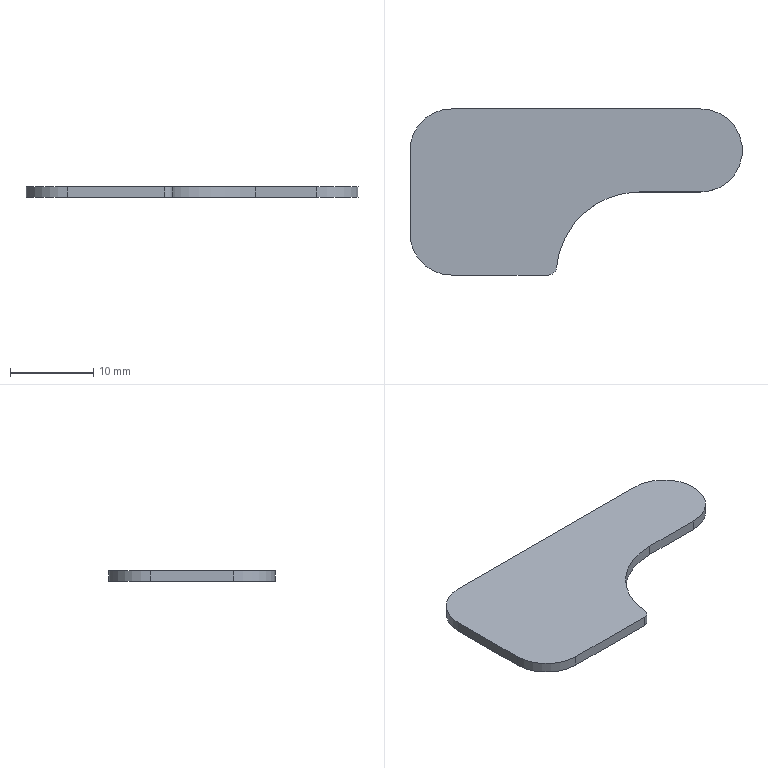Part | STEP file | gslz 2016.10.28-13_id1174_x_t | 1 solid | 11 faces | box 40 x 20 x 1.25 mm | volume 719.671 mm3 | plane 6 | cylinder 5 | commonest cylinder face diameters 10 x3 2 x1 20 x1
STEP:
#1=CARTESIAN_POINT('',(0.,0.,0.));
#2=DIRECTION('',(0.,0.,1.));
#3=DIRECTION('',(1.,0.,0.));
#4=AXIS2_PLACEMENT_3D('',#1,#2,#3);
#5=CARTESIAN_POINT('',(-1119.707,29.496,1.25));
#6=VERTEX_POINT('',#5);
#7=CARTESIAN_POINT('',(-1119.707,39.496,1.25));
#8=VERTEX_POINT('',#7);
#9=CARTESIAN_POINT('',(-1119.707,34.496,1.25));
#10=DIRECTION('',(0.,0.,1.));
#11=DIRECTION('',(-1.,0.,0.));
#12=AXIS2_PLACEMENT_3D('',#9,#10,#11);
#13=CIRCLE('',#12,5.);
#14=CARTESIAN_POINT('',(-346.108,261.5,1.25));
#15=DIRECTION('',(0.,0.,-1.));
#16=DIRECTION('',(-1.,0.,0.));
#17=AXIS2_PLACEMENT_3D('',#14,#15,#16);
#18=PLANE('',#17);
#19=CARTESIAN_POINT('',(778.599,-227.004));
#20=CARTESIAN_POINT('',(778.599,-235.664));
#21=CARTESIAN_POINT('',(771.099,-231.334));
#22=CARTESIAN_POINT('',(763.599,-227.004));
#23=CARTESIAN_POINT('',(771.099,-222.674));
#24=CARTESIAN_POINT('',(778.599,-218.344));
#25=CARTESIAN_POINT('',(778.599,-227.004));
#26=(BOUNDED_CURVE()B_SPLINE_CURVE(2,(#19,#20,#21,#22,#23,#24,#25),.UNSPECIFIED.,.T.,.F.)B_SPLINE_CURVE_WITH_KNOTS((1,2,2,2,2,1),(-2.094,0.,2.094,4.189,6.283,8.378),.UNSPECIFIED.)CURVE()GEOMETRIC_REPRESENTATION_ITEM()RATIONAL_B_SPLINE_CURVE((1.,0.5,1.,0.5,1.,0.5,1.))REPRESENTATION_ITEM(''));
#27=(GEOMETRIC_REPRESENTATION_CONTEXT(2)PARAMETRIC_REPRESENTATION_CONTEXT()REPRESENTATION_CONTEXT('',''));
#28=DEFINITIONAL_REPRESENTATION('',(#26),#27);
#29=PCURVE('',#18,#28);
#30=CARTESIAN_POINT('',(-1119.707,34.496,-2.574));
#31=DIRECTION('',(0.,0.,1.));
#32=DIRECTION('',(1.,0.,0.));
#33=AXIS2_PLACEMENT_3D('',#30,#31,#32);
#34=CYLINDRICAL_SURFACE('',#33,5.);
#35=CARTESIAN_POINT('',(3.142,3.824));
#36=DIRECTION('',(1.,0.));
#37=VECTOR('',#36,1.);
#38=LINE('',#35,#37);
#39=(GEOMETRIC_REPRESENTATION_CONTEXT(2)PARAMETRIC_REPRESENTATION_CONTEXT()REPRESENTATION_CONTEXT('',''));
#40=DEFINITIONAL_REPRESENTATION('',(#38),#39);
#41=PCURVE('',#34,#40);
#42=SURFACE_CURVE('',#13,(#29,#41),.PCURVE_S1.);
#43=EDGE_CURVE('',#6,#8,#42,.T.);
#44=ORIENTED_EDGE('',*,*,#43,.T.);
#45=CARTESIAN_POINT('',(-1149.707,39.496,1.25));
#46=VERTEX_POINT('',#45);
#47=CARTESIAN_POINT('',(-346.108,39.496,1.25));
#48=DIRECTION('',(1.,0.,0.));
#49=VECTOR('',#48,1.);
#50=LINE('',#47,#49);
#51=CARTESIAN_POINT('',(0.,-222.004));
#52=DIRECTION('',(-1.,0.));
#53=VECTOR('',#52,1.);
#54=LINE('',#51,#53);
#55=(GEOMETRIC_REPRESENTATION_CONTEXT(2)PARAMETRIC_REPRESENTATION_CONTEXT()REPRESENTATION_CONTEXT('',''));
#56=DEFINITIONAL_REPRESENTATION('',(#54),#55);
#57=PCURVE('',#18,#56);
#58=CARTESIAN_POINT('',(-1149.707,39.496,-2.574));
#59=DIRECTION('',(0.,-1.,0.));
#60=DIRECTION('',(0.,0.,-1.));
#61=AXIS2_PLACEMENT_3D('',#58,#59,#60);
#62=PLANE('',#61);
#63=CARTESIAN_POINT('',(-3.824,803.599));
#64=DIRECTION('',(0.,1.));
#65=VECTOR('',#64,1.);
#66=LINE('',#63,#65);
#67=(GEOMETRIC_REPRESENTATION_CONTEXT(2)PARAMETRIC_REPRESENTATION_CONTEXT()REPRESENTATION_CONTEXT('',''));
#68=DEFINITIONAL_REPRESENTATION('',(#66),#67);
#69=PCURVE('',#62,#68);
#70=SURFACE_CURVE('',#50,(#57,#69),.PCURVE_S1.);
#71=EDGE_CURVE('',#46,#8,#70,.T.);
#72=ORIENTED_EDGE('',*,*,#71,.F.);
#73=CARTESIAN_POINT('',(-1154.707,34.496,1.25));
#74=VERTEX_POINT('',#73);
#75=CARTESIAN_POINT('',(-1149.707,34.496,1.25));
#76=DIRECTION('',(0.,0.,1.));
#77=DIRECTION('',(-1.,0.,0.));
#78=AXIS2_PLACEMENT_3D('',#75,#76,#77);
#79=CIRCLE('',#78,5.);
#80=CARTESIAN_POINT('',(808.599,-227.004));
#81=CARTESIAN_POINT('',(808.599,-235.664));
#82=CARTESIAN_POINT('',(801.099,-231.334));
#83=CARTESIAN_POINT('',(793.599,-227.004));
#84=CARTESIAN_POINT('',(801.099,-222.674));
#85=CARTESIAN_POINT('',(808.599,-218.344));
#86=CARTESIAN_POINT('',(808.599,-227.004));
#87=(BOUNDED_CURVE()B_SPLINE_CURVE(2,(#80,#81,#82,#83,#84,#85,#86),.UNSPECIFIED.,.T.,.F.)B_SPLINE_CURVE_WITH_KNOTS((1,2,2,2,2,1),(-2.094,0.,2.094,4.189,6.283,8.378),.UNSPECIFIED.)CURVE()GEOMETRIC_REPRESENTATION_ITEM()RATIONAL_B_SPLINE_CURVE((1.,0.5,1.,0.5,1.,0.5,1.))REPRESENTATION_ITEM(''));
#88=(GEOMETRIC_REPRESENTATION_CONTEXT(2)PARAMETRIC_REPRESENTATION_CONTEXT()REPRESENTATION_CONTEXT('',''));
#89=DEFINITIONAL_REPRESENTATION('',(#87),#88);
#90=PCURVE('',#18,#89);
#91=CARTESIAN_POINT('',(-1149.707,34.496,-2.574));
#92=DIRECTION('',(0.,0.,1.));
#93=DIRECTION('',(1.,0.,0.));
#94=AXIS2_PLACEMENT_3D('',#91,#92,#93);
#95=CYLINDRICAL_SURFACE('',#94,5.);
#96=CARTESIAN_POINT('',(-3.142,3.824));
#97=DIRECTION('',(1.,0.));
#98=VECTOR('',#97,1.);
#99=LINE('',#96,#98);
#100=(GEOMETRIC_REPRESENTATION_CONTEXT(2)PARAMETRIC_REPRESENTATION_CONTEXT()REPRESENTATION_CONTEXT('',''));
#101=DEFINITIONAL_REPRESENTATION('',(#99),#100);
#102=PCURVE('',#95,#101);
#103=SURFACE_CURVE('',#79,(#90,#102),.PCURVE_S1.);
#104=EDGE_CURVE('',#46,#74,#103,.T.);
#105=ORIENTED_EDGE('',*,*,#104,.T.);
#106=CARTESIAN_POINT('',(-1154.707,24.496,1.25));
#107=VERTEX_POINT('',#106);
#108=CARTESIAN_POINT('',(-1154.707,261.5,1.25));
#109=DIRECTION('',(0.,1.,0.));
#110=VECTOR('',#109,1.);
#111=LINE('',#108,#110);
#112=CARTESIAN_POINT('',(808.599,0.));
#113=DIRECTION('',(0.,1.));
#114=VECTOR('',#113,1.);
#115=LINE('',#112,#114);
#116=(GEOMETRIC_REPRESENTATION_CONTEXT(2)PARAMETRIC_REPRESENTATION_CONTEXT()REPRESENTATION_CONTEXT('',''));
#117=DEFINITIONAL_REPRESENTATION('',(#115),#116);
#118=PCURVE('',#18,#117);
#119=CARTESIAN_POINT('',(-1154.707,24.496,-2.574));
#120=DIRECTION('',(1.,0.,0.));
#121=DIRECTION('',(0.,0.,-1.));
#122=AXIS2_PLACEMENT_3D('',#119,#120,#121);
#123=PLANE('',#122);
#124=CARTESIAN_POINT('',(-3.824,237.004));
#125=DIRECTION('',(0.,1.));
#126=VECTOR('',#125,1.);
#127=LINE('',#124,#126);
#128=(GEOMETRIC_REPRESENTATION_CONTEXT(2)PARAMETRIC_REPRESENTATION_CONTEXT()REPRESENTATION_CONTEXT('',''));
#129=DEFINITIONAL_REPRESENTATION('',(#127),#128);
#130=PCURVE('',#123,#129);
#131=SURFACE_CURVE('',#111,(#118,#130),.PCURVE_S1.);
#132=EDGE_CURVE('',#107,#74,#131,.T.);
#133=ORIENTED_EDGE('',*,*,#132,.F.);
#134=CARTESIAN_POINT('',(-1149.707,19.496,1.25));
#135=VERTEX_POINT('',#134);
#136=CARTESIAN_POINT('',(-1149.707,24.496,1.25));
#137=DIRECTION('',(0.,0.,1.));
#138=DIRECTION('',(-1.,0.,0.));
#139=AXIS2_PLACEMENT_3D('',#136,#137,#138);
#140=CIRCLE('',#139,5.);
#141=CARTESIAN_POINT('',(808.599,-237.004));
#142=CARTESIAN_POINT('',(808.599,-245.664));
#143=CARTESIAN_POINT('',(801.099,-241.334));
#144=CARTESIAN_POINT('',(793.599,-237.004));
#145=CARTESIAN_POINT('',(801.099,-232.674));
#146=CARTESIAN_POINT('',(808.599,-228.344));
#147=CARTESIAN_POINT('',(808.599,-237.004));
#148=(BOUNDED_CURVE()B_SPLINE_CURVE(2,(#141,#142,#143,#144,#145,#146,#147),.UNSPECIFIED.,.T.,.F.)B_SPLINE_CURVE_WITH_KNOTS((1,2,2,2,2,1),(-2.094,0.,2.094,4.189,6.283,8.378),.UNSPECIFIED.)CURVE()GEOMETRIC_REPRESENTATION_ITEM()RATIONAL_B_SPLINE_CURVE((1.,0.5,1.,0.5,1.,0.5,1.))REPRESENTATION_ITEM(''));
#149=(GEOMETRIC_REPRESENTATION_CONTEXT(2)PARAMETRIC_REPRESENTATION_CONTEXT()REPRESENTATION_CONTEXT('',''));
#150=DEFINITIONAL_REPRESENTATION('',(#148),#149);
#151=PCURVE('',#18,#150);
#152=CARTESIAN_POINT('',(-1149.707,24.496,-2.574));
#153=DIRECTION('',(0.,0.,1.));
#154=DIRECTION('',(1.,0.,0.));
#155=AXIS2_PLACEMENT_3D('',#152,#153,#154);
#156=CYLINDRICAL_SURFACE('',#155,5.);
#157=CARTESIAN_POINT('',(3.142,3.824));
#158=DIRECTION('',(1.,0.));
#159=VECTOR('',#158,1.);
#160=LINE('',#157,#159);
#161=(GEOMETRIC_REPRESENTATION_CONTEXT(2)PARAMETRIC_REPRESENTATION_CONTEXT()REPRESENTATION_CONTEXT('',''));
#162=DEFINITIONAL_REPRESENTATION('',(#160),#161);
#163=PCURVE('',#156,#162);
#164=SURFACE_CURVE('',#140,(#151,#163),.PCURVE_S1.);
#165=EDGE_CURVE('',#107,#135,#164,.T.);
#166=ORIENTED_EDGE('',*,*,#165,.T.);
#167=CARTESIAN_POINT('',(-1138.069,19.496,1.25));
#168=VERTEX_POINT('',#167);
#169=CARTESIAN_POINT('',(-346.108,19.496,1.25));
#170=DIRECTION('',(1.,0.,0.));
#171=VECTOR('',#170,1.);
#172=LINE('',#169,#171);
#173=CARTESIAN_POINT('',(0.,-242.004));
#174=DIRECTION('',(-1.,0.));
#175=VECTOR('',#174,1.);
#176=LINE('',#173,#175);
#177=(GEOMETRIC_REPRESENTATION_CONTEXT(2)PARAMETRIC_REPRESENTATION_CONTEXT()REPRESENTATION_CONTEXT('',''));
#178=DEFINITIONAL_REPRESENTATION('',(#176),#177);
#179=PCURVE('',#18,#178);
#180=CARTESIAN_POINT('',(-1141.069,19.496,-2.574));
#181=DIRECTION('',(0.,1.,0.));
#182=DIRECTION('',(0.,0.,1.));
#183=AXIS2_PLACEMENT_3D('',#180,#181,#182);
#184=PLANE('',#183);
#185=CARTESIAN_POINT('',(3.824,794.961));
#186=DIRECTION('',(0.,1.));
#187=VECTOR('',#186,1.);
#188=LINE('',#185,#187);
#189=(GEOMETRIC_REPRESENTATION_CONTEXT(2)PARAMETRIC_REPRESENTATION_CONTEXT()REPRESENTATION_CONTEXT('',''));
#190=DEFINITIONAL_REPRESENTATION('',(#188),#189);
#191=PCURVE('',#184,#190);
#192=SURFACE_CURVE('',#172,(#179,#191),.PCURVE_S1.);
#193=EDGE_CURVE('',#135,#168,#192,.T.);
#194=ORIENTED_EDGE('',*,*,#193,.T.);
#195=CARTESIAN_POINT('',(-1137.073,20.405,1.25));
#196=VERTEX_POINT('',#195);
#197=CARTESIAN_POINT('',(-1138.069,20.496,1.25));
#198=DIRECTION('',(0.,0.,1.));
#199=DIRECTION('',(-1.,0.,0.));
#200=AXIS2_PLACEMENT_3D('',#197,#198,#199);
#201=CIRCLE('',#200,1.);
#202=CARTESIAN_POINT('',(792.961,-241.004));
#203=CARTESIAN_POINT('',(792.961,-242.736));
#204=CARTESIAN_POINT('',(791.461,-241.87));
#205=CARTESIAN_POINT('',(789.961,-241.004));
#206=CARTESIAN_POINT('',(791.461,-240.138));
#207=CARTESIAN_POINT('',(792.961,-239.272));
#208=CARTESIAN_POINT('',(792.961,-241.004));
#209=(BOUNDED_CURVE()B_SPLINE_CURVE(2,(#202,#203,#204,#205,#206,#207,#208),.UNSPECIFIED.,.T.,.F.)B_SPLINE_CURVE_WITH_KNOTS((1,2,2,2,2,1),(-2.094,0.,2.094,4.189,6.283,8.378),.UNSPECIFIED.)CURVE()GEOMETRIC_REPRESENTATION_ITEM()RATIONAL_B_SPLINE_CURVE((1.,0.5,1.,0.5,1.,0.5,1.))REPRESENTATION_ITEM(''));
#210=(GEOMETRIC_REPRESENTATION_CONTEXT(2)PARAMETRIC_REPRESENTATION_CONTEXT()REPRESENTATION_CONTEXT('',''));
#211=DEFINITIONAL_REPRESENTATION('',(#209),#210);
#212=PCURVE('',#18,#211);
#213=CARTESIAN_POINT('',(-1138.069,20.496,-2.574));
#214=DIRECTION('',(0.,0.,1.));
#215=DIRECTION('',(1.,0.,0.));
#216=AXIS2_PLACEMENT_3D('',#213,#214,#215);
#217=CYLINDRICAL_SURFACE('',#216,1.);
#218=CARTESIAN_POINT('',(3.142,3.824));
#219=DIRECTION('',(1.,0.));
#220=VECTOR('',#219,1.);
#221=LINE('',#218,#220);
#222=(GEOMETRIC_REPRESENTATION_CONTEXT(2)PARAMETRIC_REPRESENTATION_CONTEXT()REPRESENTATION_CONTEXT('',''));
#223=DEFINITIONAL_REPRESENTATION('',(#221),#222);
#224=PCURVE('',#217,#223);
#225=SURFACE_CURVE('',#201,(#212,#224),.PCURVE_S1.);
#226=EDGE_CURVE('',#168,#196,#225,.T.);
#227=ORIENTED_EDGE('',*,*,#226,.T.);
#228=CARTESIAN_POINT('',(-1127.115,29.496,1.25));
#229=VERTEX_POINT('',#228);
#230=CARTESIAN_POINT('',(-1127.115,19.496,1.25));
#231=DIRECTION('',(0.,0.,-1.));
#232=DIRECTION('',(-1.,0.,0.));
#233=AXIS2_PLACEMENT_3D('',#230,#231,#232);
#234=CIRCLE('',#233,10.);
#235=CARTESIAN_POINT('',(781.007,-242.004));
#236=DIRECTION('',(1.,0.));
#237=AXIS2_PLACEMENT_2D('',#235,#236);
#238=CIRCLE('',#237,10.);
#239=(GEOMETRIC_REPRESENTATION_CONTEXT(2)PARAMETRIC_REPRESENTATION_CONTEXT()REPRESENTATION_CONTEXT('',''));
#240=DEFINITIONAL_REPRESENTATION('',(#238),#239);
#241=PCURVE('',#18,#240);
#242=CARTESIAN_POINT('',(-1127.115,19.496,-2.574));
#243=DIRECTION('',(0.,0.,1.));
#244=DIRECTION('',(1.,0.,0.));
#245=AXIS2_PLACEMENT_3D('',#242,#243,#244);
#246=CYLINDRICAL_SURFACE('',#245,10.);
#247=CARTESIAN_POINT('',(3.142,3.824));
#248=DIRECTION('',(-1.,0.));
#249=VECTOR('',#248,1.);
#250=LINE('',#247,#249);
#251=(GEOMETRIC_REPRESENTATION_CONTEXT(2)PARAMETRIC_REPRESENTATION_CONTEXT()REPRESENTATION_CONTEXT('',''));
#252=DEFINITIONAL_REPRESENTATION('',(#250),#251);
#253=PCURVE('',#246,#252);
#254=SURFACE_CURVE('',#234,(#241,#253),.PCURVE_S1.);
#255=EDGE_CURVE('',#196,#229,#254,.T.);
#256=ORIENTED_EDGE('',*,*,#255,.T.);
#257=CARTESIAN_POINT('',(-346.108,29.496,1.25));
#258=DIRECTION('',(-1.,0.,0.));
#259=VECTOR('',#258,1.);
#260=LINE('',#257,#259);
#261=CARTESIAN_POINT('',(0.,-232.004));
#262=DIRECTION('',(1.,0.));
#263=VECTOR('',#262,1.);
#264=LINE('',#261,#263);
#265=(GEOMETRIC_REPRESENTATION_CONTEXT(2)PARAMETRIC_REPRESENTATION_CONTEXT()REPRESENTATION_CONTEXT('',''));
#266=DEFINITIONAL_REPRESENTATION('',(#264),#265);
#267=PCURVE('',#18,#266);
#268=CARTESIAN_POINT('',(-1119.707,29.496,-2.574));
#269=DIRECTION('',(0.,1.,0.));
#270=DIRECTION('',(-1.,0.,0.));
#271=AXIS2_PLACEMENT_3D('',#268,#269,#270);
#272=PLANE('',#271);
#273=CARTESIAN_POINT('',(-773.599,3.824));
#274=DIRECTION('',(1.,0.));
#275=VECTOR('',#274,1.);
#276=LINE('',#273,#275);
#277=(GEOMETRIC_REPRESENTATION_CONTEXT(2)PARAMETRIC_REPRESENTATION_CONTEXT()REPRESENTATION_CONTEXT('',''));
#278=DEFINITIONAL_REPRESENTATION('',(#276),#277);
#279=PCURVE('',#272,#278);
#280=SURFACE_CURVE('',#260,(#267,#279),.PCURVE_S1.);
#281=EDGE_CURVE('',#6,#229,#280,.T.);
#282=ORIENTED_EDGE('',*,*,#281,.F.);
#283=EDGE_LOOP('',(#44,#72,#105,#133,#166,#194,#227,#256,#282));
#284=FACE_BOUND('',#283,.T.);
#285=ADVANCED_FACE('',(#284),#18,.F.);
#286=CARTESIAN_POINT('',(-1119.707,39.496,0.));
#287=VERTEX_POINT('',#286);
#288=CARTESIAN_POINT('',(-1149.707,39.496,0.));
#289=VERTEX_POINT('',#288);
#290=CARTESIAN_POINT('',(-346.108,39.496,0.));
#291=DIRECTION('',(-1.,0.,0.));
#292=VECTOR('',#291,1.);
#293=LINE('',#290,#292);
#294=CARTESIAN_POINT('',(-2.574,803.599));
#295=DIRECTION('',(0.,-1.));
#296=VECTOR('',#295,1.);
#297=LINE('',#294,#296);
#298=(GEOMETRIC_REPRESENTATION_CONTEXT(2)PARAMETRIC_REPRESENTATION_CONTEXT()REPRESENTATION_CONTEXT('',''));
#299=DEFINITIONAL_REPRESENTATION('',(#297),#298);
#300=PCURVE('',#62,#299);
#301=CARTESIAN_POINT('',(-346.108,261.5,0.));
#302=DIRECTION('',(0.,0.,-1.));
#303=DIRECTION('',(-1.,0.,0.));
#304=AXIS2_PLACEMENT_3D('',#301,#302,#303);
#305=PLANE('',#304);
#306=CARTESIAN_POINT('',(0.,-222.004));
#307=DIRECTION('',(1.,0.));
#308=VECTOR('',#307,1.);
#309=LINE('',#306,#308);
#310=(GEOMETRIC_REPRESENTATION_CONTEXT(2)PARAMETRIC_REPRESENTATION_CONTEXT()REPRESENTATION_CONTEXT('',''));
#311=DEFINITIONAL_REPRESENTATION('',(#309),#310);
#312=PCURVE('',#305,#311);
#313=SURFACE_CURVE('',#293,(#300,#312),.PCURVE_S1.);
#314=EDGE_CURVE('',#287,#289,#313,.T.);
#315=ORIENTED_EDGE('',*,*,#314,.T.);
#316=CARTESIAN_POINT('',(-1149.707,39.496,-2.574));
#317=DIRECTION('',(0.,0.,-1.));
#318=VECTOR('',#317,1.);
#319=LINE('',#316,#318);
#320=CARTESIAN_POINT('',(0.,0.));
#321=DIRECTION('',(1.,0.));
#322=VECTOR('',#321,1.);
#323=LINE('',#320,#322);
#324=(GEOMETRIC_REPRESENTATION_CONTEXT(2)PARAMETRIC_REPRESENTATION_CONTEXT()REPRESENTATION_CONTEXT('',''));
#325=DEFINITIONAL_REPRESENTATION('',(#323),#324);
#326=PCURVE('',#62,#325);
#327=CARTESIAN_POINT('',(1.571,0.));
#328=DIRECTION('',(0.,-1.));
#329=VECTOR('',#328,1.);
#330=LINE('',#327,#329);
#331=(GEOMETRIC_REPRESENTATION_CONTEXT(2)PARAMETRIC_REPRESENTATION_CONTEXT()REPRESENTATION_CONTEXT('',''));
#332=DEFINITIONAL_REPRESENTATION('',(#330),#331);
#333=PCURVE('',#95,#332);
#334=SURFACE_CURVE('',#319,(#326,#333),.PCURVE_S1.);
#335=EDGE_CURVE('',#46,#289,#334,.T.);
#336=ORIENTED_EDGE('',*,*,#335,.F.);
#337=ORIENTED_EDGE('',*,*,#71,.T.);
#338=CARTESIAN_POINT('',(-1119.707,39.496,-2.574));
#339=DIRECTION('',(0.,0.,-1.));
#340=VECTOR('',#339,1.);
#341=LINE('',#338,#340);
#342=CARTESIAN_POINT('',(0.,30.));
#343=DIRECTION('',(1.,0.));
#344=VECTOR('',#343,1.);
#345=LINE('',#342,#344);
#346=(GEOMETRIC_REPRESENTATION_CONTEXT(2)PARAMETRIC_REPRESENTATION_CONTEXT()REPRESENTATION_CONTEXT('',''));
#347=DEFINITIONAL_REPRESENTATION('',(#345),#346);
#348=PCURVE('',#62,#347);
#349=CARTESIAN_POINT('',(7.854,0.));
#350=DIRECTION('',(0.,-1.));
#351=VECTOR('',#350,1.);
#352=LINE('',#349,#351);
#353=(GEOMETRIC_REPRESENTATION_CONTEXT(2)PARAMETRIC_REPRESENTATION_CONTEXT()REPRESENTATION_CONTEXT('',''));
#354=DEFINITIONAL_REPRESENTATION('',(#352),#353);
#355=PCURVE('',#34,#354);
#356=SURFACE_CURVE('',#341,(#348,#355),.PCURVE_S1.);
#357=EDGE_CURVE('',#8,#287,#356,.T.);
#358=ORIENTED_EDGE('',*,*,#357,.T.);
#359=EDGE_LOOP('',(#315,#336,#337,#358));
#360=FACE_BOUND('',#359,.T.);
#361=ADVANCED_FACE('',(#360),#62,.F.);
#362=CARTESIAN_POINT('',(-1119.707,29.496,0.));
#363=VERTEX_POINT('',#362);
#364=CARTESIAN_POINT('',(-1119.707,34.496,0.));
#365=DIRECTION('',(0.,0.,1.));
#366=DIRECTION('',(-1.,0.,0.));
#367=AXIS2_PLACEMENT_3D('',#364,#365,#366);
#368=CIRCLE('',#367,5.);
#369=CARTESIAN_POINT('',(3.142,2.574));
#370=DIRECTION('',(1.,0.));
#371=VECTOR('',#370,1.);
#372=LINE('',#369,#371);
#373=(GEOMETRIC_REPRESENTATION_CONTEXT(2)PARAMETRIC_REPRESENTATION_CONTEXT()REPRESENTATION_CONTEXT('',''));
#374=DEFINITIONAL_REPRESENTATION('',(#372),#373);
#375=PCURVE('',#34,#374);
#376=CARTESIAN_POINT('',(778.599,-227.004));
#377=CARTESIAN_POINT('',(778.599,-235.664));
#378=CARTESIAN_POINT('',(771.099,-231.334));
#379=CARTESIAN_POINT('',(763.599,-227.004));
#380=CARTESIAN_POINT('',(771.099,-222.674));
#381=CARTESIAN_POINT('',(778.599,-218.344));
#382=CARTESIAN_POINT('',(778.599,-227.004));
#383=(BOUNDED_CURVE()B_SPLINE_CURVE(2,(#376,#377,#378,#379,#380,#381,#382),.UNSPECIFIED.,.T.,.F.)B_SPLINE_CURVE_WITH_KNOTS((1,2,2,2,2,1),(-2.094,0.,2.094,4.189,6.283,8.378),.UNSPECIFIED.)CURVE()GEOMETRIC_REPRESENTATION_ITEM()RATIONAL_B_SPLINE_CURVE((1.,0.5,1.,0.5,1.,0.5,1.))REPRESENTATION_ITEM(''));
#384=(GEOMETRIC_REPRESENTATION_CONTEXT(2)PARAMETRIC_REPRESENTATION_CONTEXT()REPRESENTATION_CONTEXT('',''));
#385=DEFINITIONAL_REPRESENTATION('',(#383),#384);
#386=PCURVE('',#305,#385);
#387=SURFACE_CURVE('',#368,(#375,#386),.PCURVE_S1.);
#388=EDGE_CURVE('',#363,#287,#387,.T.);
#389=ORIENTED_EDGE('',*,*,#388,.T.);
#390=ORIENTED_EDGE('',*,*,#357,.F.);
#391=ORIENTED_EDGE('',*,*,#43,.F.);
#392=CARTESIAN_POINT('',(-1119.707,29.496,-2.574));
#393=DIRECTION('',(0.,0.,-1.));
#394=VECTOR('',#393,1.);
#395=LINE('',#392,#394);
#396=CARTESIAN_POINT('',(4.712,0.));
#397=DIRECTION('',(0.,-1.));
#398=VECTOR('',#397,1.);
#399=LINE('',#396,#398);
#400=(GEOMETRIC_REPRESENTATION_CONTEXT(2)PARAMETRIC_REPRESENTATION_CONTEXT()REPRESENTATION_CONTEXT('',''));
#401=DEFINITIONAL_REPRESENTATION('',(#399),#400);
#402=PCURVE('',#34,#401);
#403=CARTESIAN_POINT('',(0.,0.));
#404=DIRECTION('',(0.,-1.));
#405=VECTOR('',#404,1.);
#406=LINE('',#403,#405);
#407=(GEOMETRIC_REPRESENTATION_CONTEXT(2)PARAMETRIC_REPRESENTATION_CONTEXT()REPRESENTATION_CONTEXT('',''));
#408=DEFINITIONAL_REPRESENTATION('',(#406),#407);
#409=PCURVE('',#272,#408);
#410=SURFACE_CURVE('',#395,(#402,#409),.PCURVE_S1.);
#411=EDGE_CURVE('',#6,#363,#410,.T.);
#412=ORIENTED_EDGE('',*,*,#411,.T.);
#413=EDGE_LOOP('',(#389,#390,#391,#412));
#414=FACE_BOUND('',#413,.T.);
#415=ADVANCED_FACE('',(#414),#34,.T.);
#416=CARTESIAN_POINT('',(-1127.115,29.496,0.));
#417=VERTEX_POINT('',#416);
#418=CARTESIAN_POINT('',(-346.108,29.496,0.));
#419=DIRECTION('',(-1.,0.,0.));
#420=VECTOR('',#419,1.);
#421=LINE('',#418,#420);
#422=CARTESIAN_POINT('',(-773.599,2.574));
#423=DIRECTION('',(1.,0.));
#424=VECTOR('',#423,1.);
#425=LINE('',#422,#424);
#426=(GEOMETRIC_REPRESENTATION_CONTEXT(2)PARAMETRIC_REPRESENTATION_CONTEXT()REPRESENTATION_CONTEXT('',''));
#427=DEFINITIONAL_REPRESENTATION('',(#425),#426);
#428=PCURVE('',#272,#427);
#429=CARTESIAN_POINT('',(0.,-232.004));
#430=DIRECTION('',(1.,0.));
#431=VECTOR('',#430,1.);
#432=LINE('',#429,#431);
#433=(GEOMETRIC_REPRESENTATION_CONTEXT(2)PARAMETRIC_REPRESENTATION_CONTEXT()REPRESENTATION_CONTEXT('',''));
#434=DEFINITIONAL_REPRESENTATION('',(#432),#433);
#435=PCURVE('',#305,#434);
#436=SURFACE_CURVE('',#421,(#428,#435),.PCURVE_S1.);
#437=EDGE_CURVE('',#363,#417,#436,.T.);
#438=ORIENTED_EDGE('',*,*,#437,.F.);
#439=ORIENTED_EDGE('',*,*,#411,.F.);
#440=ORIENTED_EDGE('',*,*,#281,.T.);
#441=CARTESIAN_POINT('',(-1127.115,29.496,-2.574));
#442=DIRECTION('',(0.,0.,-1.));
#443=VECTOR('',#442,1.);
#444=LINE('',#441,#443);
#445=CARTESIAN_POINT('',(7.408,0.));
#446=DIRECTION('',(0.,-1.));
#447=VECTOR('',#446,1.);
#448=LINE('',#445,#447);
#449=(GEOMETRIC_REPRESENTATION_CONTEXT(2)PARAMETRIC_REPRESENTATION_CONTEXT()REPRESENTATION_CONTEXT('',''));
#450=DEFINITIONAL_REPRESENTATION('',(#448),#449);
#451=PCURVE('',#272,#450);
#452=CARTESIAN_POINT('',(1.571,0.));
#453=DIRECTION('',(0.,-1.));
#454=VECTOR('',#453,1.);
#455=LINE('',#452,#454);
#456=(GEOMETRIC_REPRESENTATION_CONTEXT(2)PARAMETRIC_REPRESENTATION_CONTEXT()REPRESENTATION_CONTEXT('',''));
#457=DEFINITIONAL_REPRESENTATION('',(#455),#456);
#458=PCURVE('',#246,#457);
#459=SURFACE_CURVE('',#444,(#451,#458),.PCURVE_S1.);
#460=EDGE_CURVE('',#229,#417,#459,.T.);
#461=ORIENTED_EDGE('',*,*,#460,.T.);
#462=EDGE_LOOP('',(#438,#439,#440,#461));
#463=FACE_BOUND('',#462,.T.);
#464=ADVANCED_FACE('',(#463),#272,.F.);
#465=CARTESIAN_POINT('',(-1137.073,20.405,0.));
#466=VERTEX_POINT('',#465);
#467=CARTESIAN_POINT('',(-1137.073,20.405,-2.574));
#468=DIRECTION('',(0.,0.,-1.));
#469=VECTOR('',#468,1.);
#470=LINE('',#467,#469);
#471=CARTESIAN_POINT('',(3.051,0.));
#472=DIRECTION('',(0.,-1.));
#473=VECTOR('',#472,1.);
#474=LINE('',#471,#473);
#475=(GEOMETRIC_REPRESENTATION_CONTEXT(2)PARAMETRIC_REPRESENTATION_CONTEXT()REPRESENTATION_CONTEXT('',''));
#476=DEFINITIONAL_REPRESENTATION('',(#474),#475);
#477=PCURVE('',#246,#476);
#478=CARTESIAN_POINT('',(6.192,0.));
#479=DIRECTION('',(0.,-1.));
#480=VECTOR('',#479,1.);
#481=LINE('',#478,#480);
#482=(GEOMETRIC_REPRESENTATION_CONTEXT(2)PARAMETRIC_REPRESENTATION_CONTEXT()REPRESENTATION_CONTEXT('',''));
#483=DEFINITIONAL_REPRESENTATION('',(#481),#482);
#484=PCURVE('',#217,#483);
#485=SURFACE_CURVE('',#470,(#477,#484),.PCURVE_S1.);
#486=EDGE_CURVE('',#196,#466,#485,.T.);
#487=ORIENTED_EDGE('',*,*,#486,.F.);
#488=ORIENTED_EDGE('',*,*,#255,.T.);
#489=ORIENTED_EDGE('',*,*,#460,.T.);
#490=CARTESIAN_POINT('',(-1127.115,19.496,0.));
#491=DIRECTION('',(0.,0.,-1.));
#492=DIRECTION('',(-1.,0.,0.));
#493=AXIS2_PLACEMENT_3D('',#490,#491,#492);
#494=CIRCLE('',#493,10.);
#495=CARTESIAN_POINT('',(3.142,2.574));
#496=DIRECTION('',(-1.,0.));
#497=VECTOR('',#496,1.);
#498=LINE('',#495,#497);
#499=(GEOMETRIC_REPRESENTATION_CONTEXT(2)PARAMETRIC_REPRESENTATION_CONTEXT()REPRESENTATION_CONTEXT('',''));
#500=DEFINITIONAL_REPRESENTATION('',(#498),#499);
#501=PCURVE('',#246,#500);
#502=CARTESIAN_POINT('',(781.007,-242.004));
#503=DIRECTION('',(1.,0.));
#504=AXIS2_PLACEMENT_2D('',#502,#503);
#505=CIRCLE('',#504,10.);
#506=(GEOMETRIC_REPRESENTATION_CONTEXT(2)PARAMETRIC_REPRESENTATION_CONTEXT()REPRESENTATION_CONTEXT('',''));
#507=DEFINITIONAL_REPRESENTATION('',(#505),#506);
#508=PCURVE('',#305,#507);
#509=SURFACE_CURVE('',#494,(#501,#508),.PCURVE_S1.);
#510=EDGE_CURVE('',#466,#417,#509,.T.);
#511=ORIENTED_EDGE('',*,*,#510,.F.);
#512=EDGE_LOOP('',(#487,#488,#489,#511));
#513=FACE_BOUND('',#512,.F.);
#514=ADVANCED_FACE('',(#513),#246,.F.);
#515=CARTESIAN_POINT('',(-1138.069,19.496,0.));
#516=VERTEX_POINT('',#515);
#517=CARTESIAN_POINT('',(-1138.069,20.496,0.));
#518=DIRECTION('',(0.,0.,1.));
#519=DIRECTION('',(-1.,0.,0.));
#520=AXIS2_PLACEMENT_3D('',#517,#518,#519);
#521=CIRCLE('',#520,1.);
#522=CARTESIAN_POINT('',(3.142,2.574));
#523=DIRECTION('',(1.,0.));
#524=VECTOR('',#523,1.);
#525=LINE('',#522,#524);
#526=(GEOMETRIC_REPRESENTATION_CONTEXT(2)PARAMETRIC_REPRESENTATION_CONTEXT()REPRESENTATION_CONTEXT('',''));
#527=DEFINITIONAL_REPRESENTATION('',(#525),#526);
#528=PCURVE('',#217,#527);
#529=CARTESIAN_POINT('',(792.961,-241.004));
#530=CARTESIAN_POINT('',(792.961,-242.736));
#531=CARTESIAN_POINT('',(791.461,-241.87));
#532=CARTESIAN_POINT('',(789.961,-241.004));
#533=CARTESIAN_POINT('',(791.461,-240.138));
#534=CARTESIAN_POINT('',(792.961,-239.272));
#535=CARTESIAN_POINT('',(792.961,-241.004));
#536=(BOUNDED_CURVE()B_SPLINE_CURVE(2,(#529,#530,#531,#532,#533,#534,#535),.UNSPECIFIED.,.T.,.F.)B_SPLINE_CURVE_WITH_KNOTS((1,2,2,2,2,1),(-2.094,0.,2.094,4.189,6.283,8.378),.UNSPECIFIED.)CURVE()GEOMETRIC_REPRESENTATION_ITEM()RATIONAL_B_SPLINE_CURVE((1.,0.5,1.,0.5,1.,0.5,1.))REPRESENTATION_ITEM(''));
#537=(GEOMETRIC_REPRESENTATION_CONTEXT(2)PARAMETRIC_REPRESENTATION_CONTEXT()REPRESENTATION_CONTEXT('',''));
#538=DEFINITIONAL_REPRESENTATION('',(#536),#537);
#539=PCURVE('',#305,#538);
#540=SURFACE_CURVE('',#521,(#528,#539),.PCURVE_S1.);
#541=EDGE_CURVE('',#516,#466,#540,.T.);
#542=ORIENTED_EDGE('',*,*,#541,.T.);
#543=ORIENTED_EDGE('',*,*,#486,.F.);
#544=ORIENTED_EDGE('',*,*,#226,.F.);
#545=CARTESIAN_POINT('',(-1138.069,19.496,-2.574));
#546=DIRECTION('',(0.,0.,-1.));
#547=VECTOR('',#546,1.);
#548=LINE('',#545,#547);
#549=CARTESIAN_POINT('',(4.712,0.));
#550=DIRECTION('',(0.,-1.));
#551=VECTOR('',#550,1.);
#552=LINE('',#549,#551);
#553=(GEOMETRIC_REPRESENTATION_CONTEXT(2)PARAMETRIC_REPRESENTATION_CONTEXT()REPRESENTATION_CONTEXT('',''));
#554=DEFINITIONAL_REPRESENTATION('',(#552),#553);
#555=PCURVE('',#217,#554);
#556=CARTESIAN_POINT('',(0.,3.));
#557=DIRECTION('',(-1.,0.));
#558=VECTOR('',#557,1.);
#559=LINE('',#556,#558);
#560=(GEOMETRIC_REPRESENTATION_CONTEXT(2)PARAMETRIC_REPRESENTATION_CONTEXT()REPRESENTATION_CONTEXT('',''));
#561=DEFINITIONAL_REPRESENTATION('',(#559),#560);
#562=PCURVE('',#184,#561);
#563=SURFACE_CURVE('',#548,(#555,#562),.PCURVE_S1.);
#564=EDGE_CURVE('',#168,#516,#563,.T.);
#565=ORIENTED_EDGE('',*,*,#564,.T.);
#566=EDGE_LOOP('',(#542,#543,#544,#565));
#567=FACE_BOUND('',#566,.T.);
#568=ADVANCED_FACE('',(#567),#217,.T.);
#569=CARTESIAN_POINT('',(-1149.707,19.496,0.));
#570=VERTEX_POINT('',#569);
#571=CARTESIAN_POINT('',(-346.108,19.496,0.));
#572=DIRECTION('',(1.,0.,0.));
#573=VECTOR('',#572,1.);
#574=LINE('',#571,#573);
#575=CARTESIAN_POINT('',(2.574,794.961));
#576=DIRECTION('',(0.,1.));
#577=VECTOR('',#576,1.);
#578=LINE('',#575,#577);
#579=(GEOMETRIC_REPRESENTATION_CONTEXT(2)PARAMETRIC_REPRESENTATION_CONTEXT()REPRESENTATION_CONTEXT('',''));
#580=DEFINITIONAL_REPRESENTATION('',(#578),#579);
#581=PCURVE('',#184,#580);
#582=CARTESIAN_POINT('',(0.,-242.004));
#583=DIRECTION('',(-1.,0.));
#584=VECTOR('',#583,1.);
#585=LINE('',#582,#584);
#586=(GEOMETRIC_REPRESENTATION_CONTEXT(2)PARAMETRIC_REPRESENTATION_CONTEXT()REPRESENTATION_CONTEXT('',''));
#587=DEFINITIONAL_REPRESENTATION('',(#585),#586);
#588=PCURVE('',#305,#587);
#589=SURFACE_CURVE('',#574,(#581,#588),.PCURVE_S1.);
#590=EDGE_CURVE('',#570,#516,#589,.T.);
#591=ORIENTED_EDGE('',*,*,#590,.T.);
#592=ORIENTED_EDGE('',*,*,#564,.F.);
#593=ORIENTED_EDGE('',*,*,#193,.F.);
#594=CARTESIAN_POINT('',(-1149.707,19.496,-2.574));
#595=DIRECTION('',(0.,0.,-1.));
#596=VECTOR('',#595,1.);
#597=LINE('',#594,#596);
#598=CARTESIAN_POINT('',(0.,-8.638));
#599=DIRECTION('',(-1.,0.));
#600=VECTOR('',#599,1.);
#601=LINE('',#598,#600);
#602=(GEOMETRIC_REPRESENTATION_CONTEXT(2)PARAMETRIC_REPRESENTATION_CONTEXT()REPRESENTATION_CONTEXT('',''));
#603=DEFINITIONAL_REPRESENTATION('',(#601),#602);
#604=PCURVE('',#184,#603);
#605=CARTESIAN_POINT('',(4.712,0.));
#606=DIRECTION('',(0.,-1.));
#607=VECTOR('',#606,1.);
#608=LINE('',#605,#607);
#609=(GEOMETRIC_REPRESENTATION_CONTEXT(2)PARAMETRIC_REPRESENTATION_CONTEXT()REPRESENTATION_CONTEXT('',''));
#610=DEFINITIONAL_REPRESENTATION('',(#608),#609);
#611=PCURVE('',#156,#610);
#612=SURFACE_CURVE('',#597,(#604,#611),.PCURVE_S1.);
#613=EDGE_CURVE('',#135,#570,#612,.T.);
#614=ORIENTED_EDGE('',*,*,#613,.T.);
#615=EDGE_LOOP('',(#591,#592,#593,#614));
#616=FACE_BOUND('',#615,.T.);
#617=ADVANCED_FACE('',(#616),#184,.F.);
#618=CARTESIAN_POINT('',(-1154.707,24.496,0.));
#619=VERTEX_POINT('',#618);
#620=CARTESIAN_POINT('',(-1149.707,24.496,0.));
#621=DIRECTION('',(0.,0.,1.));
#622=DIRECTION('',(-1.,0.,0.));
#623=AXIS2_PLACEMENT_3D('',#620,#621,#622);
#624=CIRCLE('',#623,5.);
#625=CARTESIAN_POINT('',(3.142,2.574));
#626=DIRECTION('',(1.,0.));
#627=VECTOR('',#626,1.);
#628=LINE('',#625,#627);
#629=(GEOMETRIC_REPRESENTATION_CONTEXT(2)PARAMETRIC_REPRESENTATION_CONTEXT()REPRESENTATION_CONTEXT('',''));
#630=DEFINITIONAL_REPRESENTATION('',(#628),#629);
#631=PCURVE('',#156,#630);
#632=CARTESIAN_POINT('',(808.599,-237.004));
#633=CARTESIAN_POINT('',(808.599,-245.664));
#634=CARTESIAN_POINT('',(801.099,-241.334));
#635=CARTESIAN_POINT('',(793.599,-237.004));
#636=CARTESIAN_POINT('',(801.099,-232.674));
#637=CARTESIAN_POINT('',(808.599,-228.344));
#638=CARTESIAN_POINT('',(808.599,-237.004));
#639=(BOUNDED_CURVE()B_SPLINE_CURVE(2,(#632,#633,#634,#635,#636,#637,#638),.UNSPECIFIED.,.T.,.F.)B_SPLINE_CURVE_WITH_KNOTS((1,2,2,2,2,1),(-2.094,0.,2.094,4.189,6.283,8.378),.UNSPECIFIED.)CURVE()GEOMETRIC_REPRESENTATION_ITEM()RATIONAL_B_SPLINE_CURVE((1.,0.5,1.,0.5,1.,0.5,1.))REPRESENTATION_ITEM(''));
#640=(GEOMETRIC_REPRESENTATION_CONTEXT(2)PARAMETRIC_REPRESENTATION_CONTEXT()REPRESENTATION_CONTEXT('',''));
#641=DEFINITIONAL_REPRESENTATION('',(#639),#640);
#642=PCURVE('',#305,#641);
#643=SURFACE_CURVE('',#624,(#631,#642),.PCURVE_S1.);
#644=EDGE_CURVE('',#619,#570,#643,.T.);
#645=ORIENTED_EDGE('',*,*,#644,.T.);
#646=ORIENTED_EDGE('',*,*,#613,.F.);
#647=ORIENTED_EDGE('',*,*,#165,.F.);
#648=CARTESIAN_POINT('',(-1154.707,24.496,-2.574));
#649=DIRECTION('',(0.,0.,-1.));
#650=VECTOR('',#649,1.);
#651=LINE('',#648,#650);
#652=CARTESIAN_POINT('',(3.142,0.));
#653=DIRECTION('',(0.,-1.));
#654=VECTOR('',#653,1.);
#655=LINE('',#652,#654);
#656=(GEOMETRIC_REPRESENTATION_CONTEXT(2)PARAMETRIC_REPRESENTATION_CONTEXT()REPRESENTATION_CONTEXT('',''));
#657=DEFINITIONAL_REPRESENTATION('',(#655),#656);
#658=PCURVE('',#156,#657);
#659=CARTESIAN_POINT('',(0.,0.));
#660=DIRECTION('',(1.,0.));
#661=VECTOR('',#660,1.);
#662=LINE('',#659,#661);
#663=(GEOMETRIC_REPRESENTATION_CONTEXT(2)PARAMETRIC_REPRESENTATION_CONTEXT()REPRESENTATION_CONTEXT('',''));
#664=DEFINITIONAL_REPRESENTATION('',(#662),#663);
#665=PCURVE('',#123,#664);
#666=SURFACE_CURVE('',#651,(#658,#665),.PCURVE_S1.);
#667=EDGE_CURVE('',#107,#619,#666,.T.);
#668=ORIENTED_EDGE('',*,*,#667,.T.);
#669=EDGE_LOOP('',(#645,#646,#647,#668));
#670=FACE_BOUND('',#669,.T.);
#671=ADVANCED_FACE('',(#670),#156,.T.);
#672=CARTESIAN_POINT('',(-1154.707,34.496,0.));
#673=VERTEX_POINT('',#672);
#674=CARTESIAN_POINT('',(-1154.707,261.5,0.));
#675=DIRECTION('',(0.,-1.,0.));
#676=VECTOR('',#675,1.);
#677=LINE('',#674,#676);
#678=CARTESIAN_POINT('',(-2.574,237.004));
#679=DIRECTION('',(0.,-1.));
#680=VECTOR('',#679,1.);
#681=LINE('',#678,#680);
#682=(GEOMETRIC_REPRESENTATION_CONTEXT(2)PARAMETRIC_REPRESENTATION_CONTEXT()REPRESENTATION_CONTEXT('',''));
#683=DEFINITIONAL_REPRESENTATION('',(#681),#682);
#684=PCURVE('',#123,#683);
#685=CARTESIAN_POINT('',(808.599,0.));
#686=DIRECTION('',(0.,-1.));
#687=VECTOR('',#686,1.);
#688=LINE('',#685,#687);
#689=(GEOMETRIC_REPRESENTATION_CONTEXT(2)PARAMETRIC_REPRESENTATION_CONTEXT()REPRESENTATION_CONTEXT('',''));
#690=DEFINITIONAL_REPRESENTATION('',(#688),#689);
#691=PCURVE('',#305,#690);
#692=SURFACE_CURVE('',#677,(#684,#691),.PCURVE_S1.);
#693=EDGE_CURVE('',#673,#619,#692,.T.);
#694=ORIENTED_EDGE('',*,*,#693,.T.);
#695=ORIENTED_EDGE('',*,*,#667,.F.);
#696=ORIENTED_EDGE('',*,*,#132,.T.);
#697=CARTESIAN_POINT('',(-1154.707,34.496,-2.574));
#698=DIRECTION('',(0.,0.,-1.));
#699=VECTOR('',#698,1.);
#700=LINE('',#697,#699);
#701=CARTESIAN_POINT('',(0.,10.));
#702=DIRECTION('',(1.,0.));
#703=VECTOR('',#702,1.);
#704=LINE('',#701,#703);
#705=(GEOMETRIC_REPRESENTATION_CONTEXT(2)PARAMETRIC_REPRESENTATION_CONTEXT()REPRESENTATION_CONTEXT('',''));
#706=DEFINITIONAL_REPRESENTATION('',(#704),#705);
#707=PCURVE('',#123,#706);
#708=CARTESIAN_POINT('',(3.142,0.));
#709=DIRECTION('',(0.,-1.));
#710=VECTOR('',#709,1.);
#711=LINE('',#708,#710);
#712=(GEOMETRIC_REPRESENTATION_CONTEXT(2)PARAMETRIC_REPRESENTATION_CONTEXT()REPRESENTATION_CONTEXT('',''));
#713=DEFINITIONAL_REPRESENTATION('',(#711),#712);
#714=PCURVE('',#95,#713);
#715=SURFACE_CURVE('',#700,(#707,#714),.PCURVE_S1.);
#716=EDGE_CURVE('',#74,#673,#715,.T.);
#717=ORIENTED_EDGE('',*,*,#716,.T.);
#718=EDGE_LOOP('',(#694,#695,#696,#717));
#719=FACE_BOUND('',#718,.T.);
#720=ADVANCED_FACE('',(#719),#123,.F.);
#721=CARTESIAN_POINT('',(-1149.707,34.496,0.));
#722=DIRECTION('',(0.,0.,1.));
#723=DIRECTION('',(-1.,0.,0.));
#724=AXIS2_PLACEMENT_3D('',#721,#722,#723);
#725=CIRCLE('',#724,5.);
#726=CARTESIAN_POINT('',(-3.142,2.574));
#727=DIRECTION('',(1.,0.));
#728=VECTOR('',#727,1.);
#729=LINE('',#726,#728);
#730=(GEOMETRIC_REPRESENTATION_CONTEXT(2)PARAMETRIC_REPRESENTATION_CONTEXT()REPRESENTATION_CONTEXT('',''));
#731=DEFINITIONAL_REPRESENTATION('',(#729),#730);
#732=PCURVE('',#95,#731);
#733=CARTESIAN_POINT('',(808.599,-227.004));
#734=CARTESIAN_POINT('',(808.599,-235.664));
#735=CARTESIAN_POINT('',(801.099,-231.334));
#736=CARTESIAN_POINT('',(793.599,-227.004));
#737=CARTESIAN_POINT('',(801.099,-222.674));
#738=CARTESIAN_POINT('',(808.599,-218.344));
#739=CARTESIAN_POINT('',(808.599,-227.004));
#740=(BOUNDED_CURVE()B_SPLINE_CURVE(2,(#733,#734,#735,#736,#737,#738,#739),.UNSPECIFIED.,.T.,.F.)B_SPLINE_CURVE_WITH_KNOTS((1,2,2,2,2,1),(-2.094,0.,2.094,4.189,6.283,8.378),.UNSPECIFIED.)CURVE()GEOMETRIC_REPRESENTATION_ITEM()RATIONAL_B_SPLINE_CURVE((1.,0.5,1.,0.5,1.,0.5,1.))REPRESENTATION_ITEM(''));
#741=(GEOMETRIC_REPRESENTATION_CONTEXT(2)PARAMETRIC_REPRESENTATION_CONTEXT()REPRESENTATION_CONTEXT('',''));
#742=DEFINITIONAL_REPRESENTATION('',(#740),#741);
#743=PCURVE('',#305,#742);
#744=SURFACE_CURVE('',#725,(#732,#743),.PCURVE_S1.);
#745=EDGE_CURVE('',#289,#673,#744,.T.);
#746=ORIENTED_EDGE('',*,*,#745,.T.);
#747=ORIENTED_EDGE('',*,*,#716,.F.);
#748=ORIENTED_EDGE('',*,*,#104,.F.);
#749=ORIENTED_EDGE('',*,*,#335,.T.);
#750=EDGE_LOOP('',(#746,#747,#748,#749));
#751=FACE_BOUND('',#750,.T.);
#752=ADVANCED_FACE('',(#751),#95,.T.);
#753=ORIENTED_EDGE('',*,*,#314,.F.);
#754=ORIENTED_EDGE('',*,*,#388,.F.);
#755=ORIENTED_EDGE('',*,*,#437,.T.);
#756=ORIENTED_EDGE('',*,*,#510,.F.);
#757=ORIENTED_EDGE('',*,*,#541,.F.);
#758=ORIENTED_EDGE('',*,*,#590,.F.);
#759=ORIENTED_EDGE('',*,*,#644,.F.);
#760=ORIENTED_EDGE('',*,*,#693,.F.);
#761=ORIENTED_EDGE('',*,*,#745,.F.);
#762=EDGE_LOOP('',(#753,#754,#755,#756,#757,#758,#759,#760,#761));
#763=FACE_BOUND('',#762,.T.);
#764=ADVANCED_FACE('',(#763),#305,.T.);
#765=CLOSED_SHELL('',(#285,#361,#415,#464,#514,#568,#617,#671,#720,#752,#764));
#766=MANIFOLD_SOLID_BREP('',#765);
#767=(LENGTH_UNIT()NAMED_UNIT(*)SI_UNIT(.MILLI.,.METRE.));
#768=UNCERTAINTY_MEASURE_WITH_UNIT(LENGTH_MEASURE(0.0000001),#767,'','');
#769=(NAMED_UNIT(*)PLANE_ANGLE_UNIT()SI_UNIT($,.RADIAN.));
#770=(NAMED_UNIT(*)SI_UNIT($,.STERADIAN.)SOLID_ANGLE_UNIT());
#771=(GEOMETRIC_REPRESENTATION_CONTEXT(3)GLOBAL_UNCERTAINTY_ASSIGNED_CONTEXT((#768))GLOBAL_UNIT_ASSIGNED_CONTEXT((#767,#769,#770))REPRESENTATION_CONTEXT('',''));
#772=ADVANCED_BREP_SHAPE_REPRESENTATION('',(#4,#766),#771);